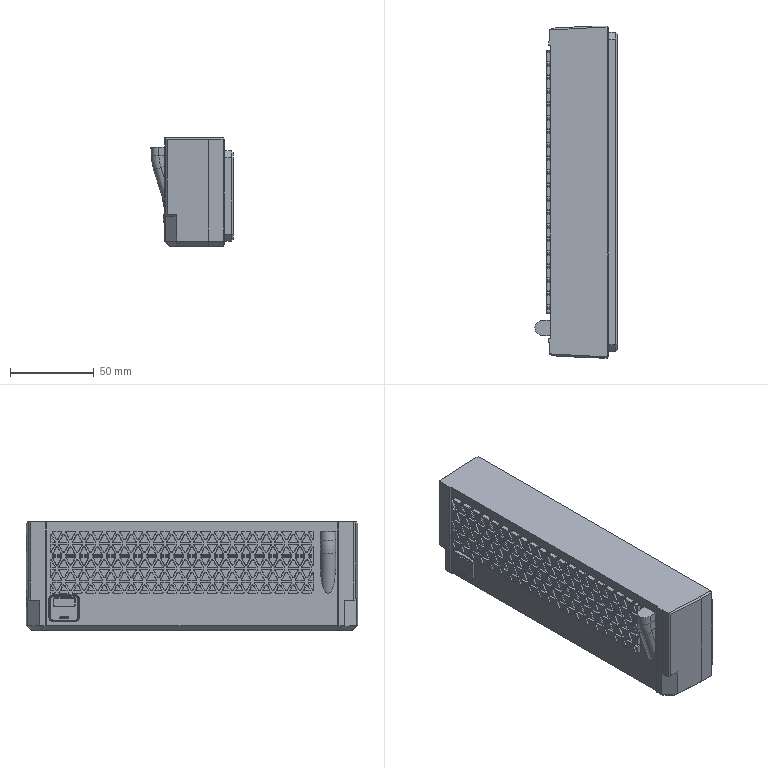Part | Creo | 1 solid | 1934 faces | box 49.15 x 198.6 x 64.721 mm | volume 475627 mm3 | spline 791 | plane 580 | cone 439 | other 68 | cylinder 51 | torus 5 | commonest cylinder face diameters 8 x30 0.4 x4 0.402 x4 0.904 x2 2.01 x2 2.9 x2